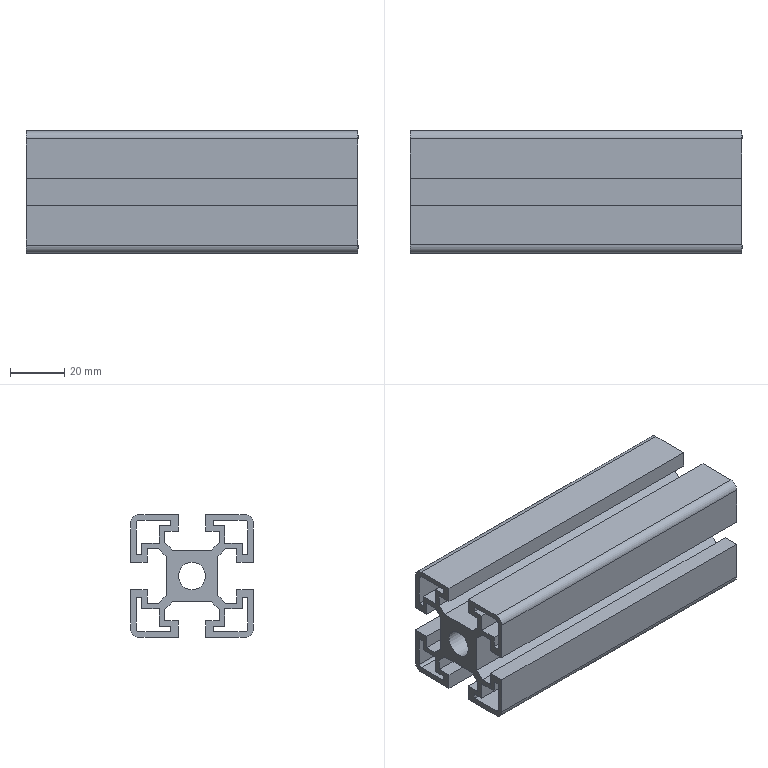Part | STEP file | bosch_3842990520_bbw6j7b49i4caf90m9u0fayle | 1 solid | 87 faces | box 122 x 45 x 45 mm | volume 99765 mm3 | plane 78 | cylinder 9 | commonest cylinder face diameters 2 x4 6 x4 10 x1